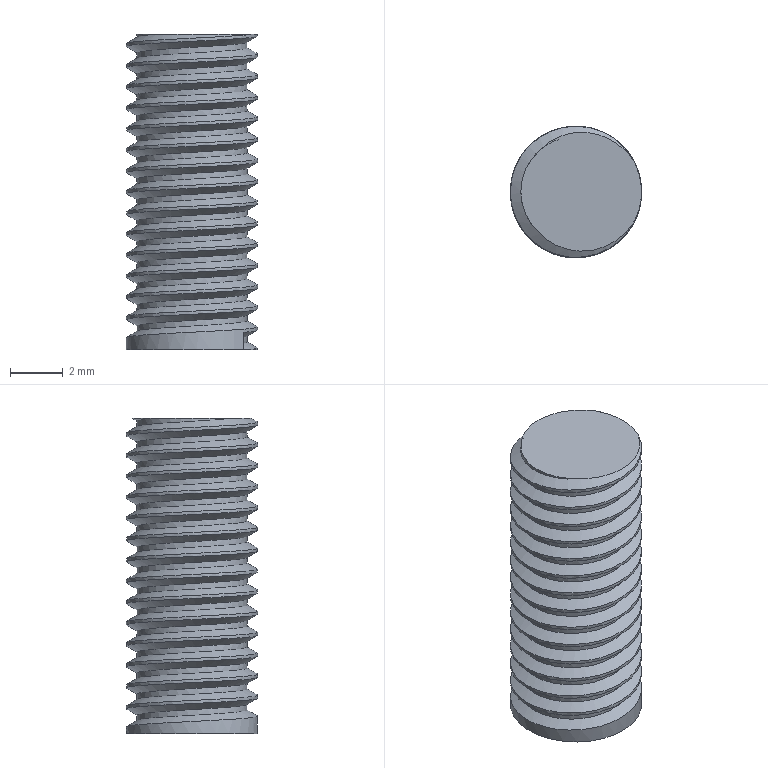Part | NX | features CYLINDER 1, DATUM_CSYS 1, THREADS 1 | 1 solid | 7 faces | box 5 x 5 x 12 mm | volume 202.074 mm3 | plane 3 | cylinder 2 | spline 2 | commonest cylinder face diameters 4.2 x1 5 x1